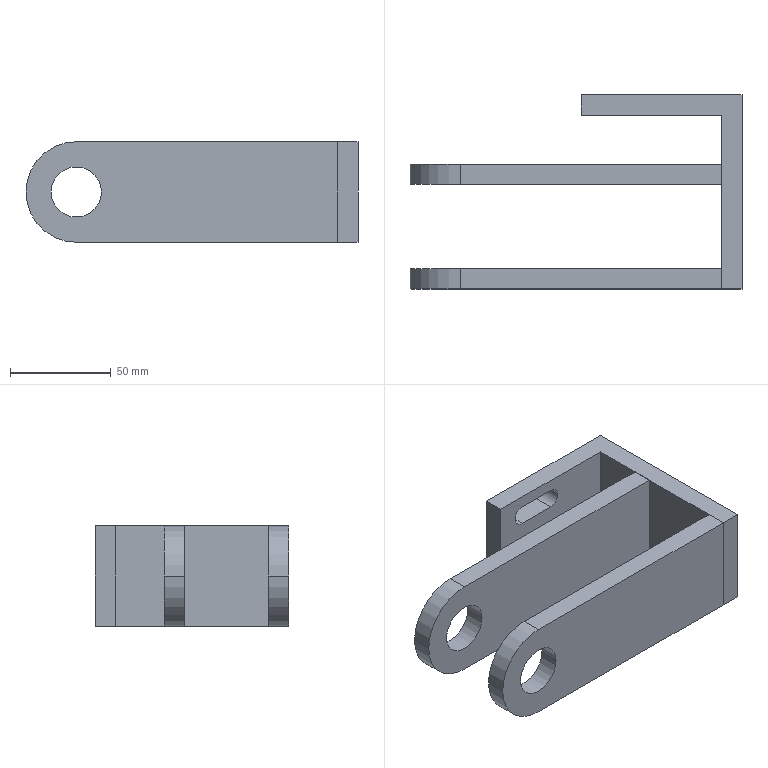Part | SolidWorks | features MoveFace 6, ICE 4, MoveCopyBody 2, Extrusion 1, MirrorSolid 1, Split 1 | 3 solids | 34 faces | box 165 x 96.4 x 50 mm | volume 217447 mm3 | plane 22 | cylinder 12 | commonest cylinder face diameters 10 x4 25 x4 50 x4
STEP:
#1=CARTESIAN_POINT('',(-87.5,-75.,37.));
#2=VERTEX_POINT('',#1);
#3=CARTESIAN_POINT('',(-62.5,-75.,37.));
#4=VERTEX_POINT('',#3);
#5=CARTESIAN_POINT('',(-75.,-75.,37.));
#6=DIRECTION('',(0.,1.,0.));
#7=DIRECTION('',(1.,0.,0.));
#8=AXIS2_PLACEMENT_3D('',#5,#6,#7);
#9=CIRCLE('',#8,12.5);
#10=EDGE_CURVE('',#2,#4,#9,.T.);
#11=ORIENTED_EDGE('',*,*,#10,.T.);
#12=CARTESIAN_POINT('',(-62.5,-85.,37.));
#13=VERTEX_POINT('',#12);
#14=CARTESIAN_POINT('',(-62.5,-75.,37.));
#15=DIRECTION('',(0.,-1.,0.));
#16=VECTOR('',#15,1000.);
#17=LINE('',#14,#16);
#18=EDGE_CURVE('',#4,#13,#17,.T.);
#19=ORIENTED_EDGE('',*,*,#18,.T.);
#20=CARTESIAN_POINT('',(-87.5,-85.,37.));
#21=VERTEX_POINT('',#20);
#22=CARTESIAN_POINT('',(-75.,-85.,37.));
#23=DIRECTION('',(0.,1.,0.));
#24=DIRECTION('',(1.,0.,0.));
#25=AXIS2_PLACEMENT_3D('',#22,#23,#24);
#26=CIRCLE('',#25,12.5);
#27=EDGE_CURVE('',#21,#13,#26,.T.);
#28=ORIENTED_EDGE('',*,*,#27,.F.);
#29=CARTESIAN_POINT('',(-87.5,-75.,37.));
#30=DIRECTION('',(0.,-1.,0.));
#31=VECTOR('',#30,1000.);
#32=LINE('',#29,#31);
#33=EDGE_CURVE('',#2,#21,#32,.T.);
#34=ORIENTED_EDGE('',*,*,#33,.F.);
#35=EDGE_LOOP('',(#11,#19,#28,#34));
#36=FACE_OUTER_BOUND('',#35,.T.);
#37=CARTESIAN_POINT('',(-75.,-75.,37.));
#38=DIRECTION('',(0.,-1.,0.));
#39=DIRECTION('',(-1.,0.,0.));
#40=AXIS2_PLACEMENT_3D('',#37,#38,#39);
#41=CYLINDRICAL_SURFACE('',#40,12.5);
#42=ADVANCED_FACE('',(#36),#41,.F.);
#43=CARTESIAN_POINT('',(-100.,-75.,37.));
#44=VERTEX_POINT('',#43);
#45=CARTESIAN_POINT('',(-75.,-75.,62.));
#46=VERTEX_POINT('',#45);
#47=CARTESIAN_POINT('',(-75.,-75.,37.));
#48=DIRECTION('',(0.,1.,0.));
#49=DIRECTION('',(1.,0.,0.));
#50=AXIS2_PLACEMENT_3D('',#47,#48,#49);
#51=CIRCLE('',#50,25.);
#52=EDGE_CURVE('',#44,#46,#51,.T.);
#53=ORIENTED_EDGE('',*,*,#52,.F.);
#54=CARTESIAN_POINT('',(-100.,-85.,37.));
#55=VERTEX_POINT('',#54);
#56=CARTESIAN_POINT('',(-100.,-75.,37.));
#57=DIRECTION('',(0.,-1.,0.));
#58=VECTOR('',#57,1000.);
#59=LINE('',#56,#58);
#60=EDGE_CURVE('',#44,#55,#59,.T.);
#61=ORIENTED_EDGE('',*,*,#60,.T.);
#62=CARTESIAN_POINT('',(-75.,-85.,62.));
#63=VERTEX_POINT('',#62);
#64=CARTESIAN_POINT('',(-75.,-85.,37.));
#65=DIRECTION('',(0.,1.,0.));
#66=DIRECTION('',(1.,0.,0.));
#67=AXIS2_PLACEMENT_3D('',#64,#65,#66);
#68=CIRCLE('',#67,25.);
#69=EDGE_CURVE('',#55,#63,#68,.T.);
#70=ORIENTED_EDGE('',*,*,#69,.T.);
#71=CARTESIAN_POINT('',(-75.,-75.,62.));
#72=DIRECTION('',(0.,-1.,0.));
#73=VECTOR('',#72,1000.);
#74=LINE('',#71,#73);
#75=EDGE_CURVE('',#46,#63,#74,.T.);
#76=ORIENTED_EDGE('',*,*,#75,.F.);
#77=EDGE_LOOP('',(#53,#61,#70,#76));
#78=FACE_OUTER_BOUND('',#77,.T.);
#79=CARTESIAN_POINT('',(-75.,-75.,37.));
#80=DIRECTION('',(0.,-1.,0.));
#81=DIRECTION('',(-1.,0.,0.));
#82=AXIS2_PLACEMENT_3D('',#79,#80,#81);
#83=CYLINDRICAL_SURFACE('',#82,25.);
#84=ADVANCED_FACE('',(#78),#83,.T.);
#85=CARTESIAN_POINT('',(55.,-85.,12.));
#86=VERTEX_POINT('',#85);
#87=CARTESIAN_POINT('',(55.,-85.,62.));
#88=VERTEX_POINT('',#87);
#89=CARTESIAN_POINT('',(55.,-85.,37.));
#90=DIRECTION('',(0.,0.,1.));
#91=VECTOR('',#90,1000.);
#92=LINE('',#89,#91);
#93=EDGE_CURVE('',#86,#88,#92,.T.);
#94=ORIENTED_EDGE('',*,*,#93,.F.);
#95=CARTESIAN_POINT('',(55.,-75.,12.));
#96=VERTEX_POINT('',#95);
#97=CARTESIAN_POINT('',(55.,-75.,12.));
#98=DIRECTION('',(0.,-1.,0.));
#99=VECTOR('',#98,1000.);
#100=LINE('',#97,#99);
#101=EDGE_CURVE('',#96,#86,#100,.T.);
#102=ORIENTED_EDGE('',*,*,#101,.F.);
#103=CARTESIAN_POINT('',(55.,-75.,62.));
#104=VERTEX_POINT('',#103);
#105=CARTESIAN_POINT('',(55.,-75.,37.));
#106=DIRECTION('',(0.,0.,1.));
#107=VECTOR('',#106,1000.);
#108=LINE('',#105,#107);
#109=EDGE_CURVE('',#96,#104,#108,.T.);
#110=ORIENTED_EDGE('',*,*,#109,.T.);
#111=CARTESIAN_POINT('',(55.,-75.,62.));
#112=DIRECTION('',(0.,1.,0.));
#113=VECTOR('',#112,1000.);
#114=LINE('',#111,#113);
#115=EDGE_CURVE('',#88,#104,#114,.T.);
#116=ORIENTED_EDGE('',*,*,#115,.F.);
#117=EDGE_LOOP('',(#94,#102,#110,#116));
#118=FACE_OUTER_BOUND('',#117,.T.);
#119=CARTESIAN_POINT('',(55.,-85.,-28.));
#120=DIRECTION('',(-1.,0.,0.));
#121=DIRECTION('',(0.,1.,0.));
#122=AXIS2_PLACEMENT_3D('',#119,#120,#121);
#123=PLANE('',#122);
#124=ADVANCED_FACE('',(#118),#123,.F.);
#125=CARTESIAN_POINT('',(-75.,-85.,12.));
#126=VERTEX_POINT('',#125);
#127=CARTESIAN_POINT('',(0.,-85.,12.));
#128=DIRECTION('',(1.,0.,0.));
#129=VECTOR('',#128,1000.);
#130=LINE('',#127,#129);
#131=EDGE_CURVE('',#126,#86,#130,.T.);
#132=ORIENTED_EDGE('',*,*,#131,.T.);
#133=ORIENTED_EDGE('',*,*,#93,.T.);
#134=CARTESIAN_POINT('',(0.,-85.,62.));
#135=DIRECTION('',(1.,0.,0.));
#136=VECTOR('',#135,1000.);
#137=LINE('',#134,#136);
#138=EDGE_CURVE('',#63,#88,#137,.T.);
#139=ORIENTED_EDGE('',*,*,#138,.F.);
#140=ORIENTED_EDGE('',*,*,#69,.F.);
#141=CARTESIAN_POINT('',(-75.,-85.,37.));
#142=DIRECTION('',(0.,1.,0.));
#143=DIRECTION('',(1.,0.,0.));
#144=AXIS2_PLACEMENT_3D('',#141,#142,#143);
#145=CIRCLE('',#144,25.);
#146=EDGE_CURVE('',#126,#55,#145,.T.);
#147=ORIENTED_EDGE('',*,*,#146,.F.);
#148=EDGE_LOOP('',(#132,#133,#139,#140,#147));
#149=FACE_OUTER_BOUND('',#148,.T.);
#150=ORIENTED_EDGE('',*,*,#27,.T.);
#151=CARTESIAN_POINT('',(-75.,-85.,37.));
#152=DIRECTION('',(0.,1.,0.));
#153=DIRECTION('',(1.,0.,0.));
#154=AXIS2_PLACEMENT_3D('',#151,#152,#153);
#155=CIRCLE('',#154,12.5);
#156=EDGE_CURVE('',#13,#21,#155,.T.);
#157=ORIENTED_EDGE('',*,*,#156,.T.);
#158=EDGE_LOOP('',(#150,#157));
#159=FACE_BOUND('',#158,.T.);
#160=CARTESIAN_POINT('',(0.,-85.,37.));
#161=DIRECTION('',(0.,1.,0.));
#162=DIRECTION('',(1.,0.,0.));
#163=AXIS2_PLACEMENT_3D('',#160,#161,#162);
#164=PLANE('',#163);
#165=ADVANCED_FACE('',(#149,#159),#164,.F.);
#166=CARTESIAN_POINT('',(0.,-75.,62.));
#167=DIRECTION('',(1.,0.,0.));
#168=VECTOR('',#167,1000.);
#169=LINE('',#166,#168);
#170=EDGE_CURVE('',#46,#104,#169,.T.);
#171=ORIENTED_EDGE('',*,*,#170,.T.);
#172=ORIENTED_EDGE('',*,*,#109,.F.);
#173=CARTESIAN_POINT('',(-75.,-75.,12.));
#174=VERTEX_POINT('',#173);
#175=CARTESIAN_POINT('',(0.,-75.,12.));
#176=DIRECTION('',(1.,0.,0.));
#177=VECTOR('',#176,1000.);
#178=LINE('',#175,#177);
#179=EDGE_CURVE('',#174,#96,#178,.T.);
#180=ORIENTED_EDGE('',*,*,#179,.F.);
#181=CARTESIAN_POINT('',(-75.,-75.,37.));
#182=DIRECTION('',(0.,1.,0.));
#183=DIRECTION('',(1.,0.,0.));
#184=AXIS2_PLACEMENT_3D('',#181,#182,#183);
#185=CIRCLE('',#184,25.);
#186=EDGE_CURVE('',#174,#44,#185,.T.);
#187=ORIENTED_EDGE('',*,*,#186,.T.);
#188=ORIENTED_EDGE('',*,*,#52,.T.);
#189=EDGE_LOOP('',(#171,#172,#180,#187,#188));
#190=FACE_OUTER_BOUND('',#189,.T.);
#191=ORIENTED_EDGE('',*,*,#10,.F.);
#192=CARTESIAN_POINT('',(-75.,-75.,37.));
#193=DIRECTION('',(0.,1.,0.));
#194=DIRECTION('',(1.,0.,0.));
#195=AXIS2_PLACEMENT_3D('',#192,#193,#194);
#196=CIRCLE('',#195,12.5);
#197=EDGE_CURVE('',#4,#2,#196,.T.);
#198=ORIENTED_EDGE('',*,*,#197,.F.);
#199=EDGE_LOOP('',(#191,#198));
#200=FACE_BOUND('',#199,.T.);
#201=CARTESIAN_POINT('',(0.,-75.,37.));
#202=DIRECTION('',(0.,1.,0.));
#203=DIRECTION('',(1.,0.,0.));
#204=AXIS2_PLACEMENT_3D('',#201,#202,#203);
#205=PLANE('',#204);
#206=ADVANCED_FACE('',(#190,#200),#205,.T.);
#207=ORIENTED_EDGE('',*,*,#18,.F.);
#208=ORIENTED_EDGE('',*,*,#197,.T.);
#209=ORIENTED_EDGE('',*,*,#33,.T.);
#210=ORIENTED_EDGE('',*,*,#156,.F.);
#211=EDGE_LOOP('',(#207,#208,#209,#210));
#212=FACE_OUTER_BOUND('',#211,.T.);
#213=CARTESIAN_POINT('',(-75.,-75.,37.));
#214=DIRECTION('',(0.,-1.,0.));
#215=DIRECTION('',(-1.,0.,0.));
#216=AXIS2_PLACEMENT_3D('',#213,#214,#215);
#217=CYLINDRICAL_SURFACE('',#216,12.5);
#218=ADVANCED_FACE('',(#212),#217,.F.);
#219=ORIENTED_EDGE('',*,*,#60,.F.);
#220=ORIENTED_EDGE('',*,*,#186,.F.);
#221=CARTESIAN_POINT('',(-75.,-75.,12.));
#222=DIRECTION('',(0.,-1.,0.));
#223=VECTOR('',#222,1000.);
#224=LINE('',#221,#223);
#225=EDGE_CURVE('',#174,#126,#224,.T.);
#226=ORIENTED_EDGE('',*,*,#225,.T.);
#227=ORIENTED_EDGE('',*,*,#146,.T.);
#228=EDGE_LOOP('',(#219,#220,#226,#227));
#229=FACE_OUTER_BOUND('',#228,.T.);
#230=CARTESIAN_POINT('',(-75.,-75.,37.));
#231=DIRECTION('',(0.,-1.,0.));
#232=DIRECTION('',(-1.,0.,0.));
#233=AXIS2_PLACEMENT_3D('',#230,#231,#232);
#234=CYLINDRICAL_SURFACE('',#233,25.);
#235=ADVANCED_FACE('',(#229),#234,.T.);
#236=ORIENTED_EDGE('',*,*,#131,.F.);
#237=ORIENTED_EDGE('',*,*,#225,.F.);
#238=ORIENTED_EDGE('',*,*,#179,.T.);
#239=ORIENTED_EDGE('',*,*,#101,.T.);
#240=EDGE_LOOP('',(#236,#237,#238,#239));
#241=FACE_OUTER_BOUND('',#240,.T.);
#242=CARTESIAN_POINT('',(0.,-75.,12.));
#243=DIRECTION('',(0.,0.,-1.));
#244=DIRECTION('',(-1.,0.,0.));
#245=AXIS2_PLACEMENT_3D('',#242,#243,#244);
#246=PLANE('',#245);
#247=ADVANCED_FACE('',(#241),#246,.T.);
#248=ORIENTED_EDGE('',*,*,#138,.T.);
#249=ORIENTED_EDGE('',*,*,#115,.T.);
#250=ORIENTED_EDGE('',*,*,#170,.F.);
#251=ORIENTED_EDGE('',*,*,#75,.T.);
#252=EDGE_LOOP('',(#248,#249,#250,#251));
#253=FACE_OUTER_BOUND('',#252,.T.);
#254=CARTESIAN_POINT('',(0.,-75.,62.));
#255=DIRECTION('',(0.,0.,-1.));
#256=DIRECTION('',(-1.,0.,0.));
#257=AXIS2_PLACEMENT_3D('',#254,#255,#256);
#258=PLANE('',#257);
#259=ADVANCED_FACE('',(#253),#258,.F.);
#260=CLOSED_SHELL('',(#42,#84,#124,#165,#206,#218,#235,#247,#259));
#261=MANIFOLD_SOLID_BREP('',#260);
#262=CARTESIAN_POINT('',(-75.,-33.,12.));
#263=VERTEX_POINT('',#262);
#264=CARTESIAN_POINT('',(-100.,-33.,37.));
#265=VERTEX_POINT('',#264);
#266=CARTESIAN_POINT('',(-75.,-33.,37.));
#267=DIRECTION('',(0.,1.,0.));
#268=DIRECTION('',(1.,0.,0.));
#269=AXIS2_PLACEMENT_3D('',#266,#267,#268);
#270=CIRCLE('',#269,25.);
#271=EDGE_CURVE('',#263,#265,#270,.T.);
#272=ORIENTED_EDGE('',*,*,#271,.T.);
#273=CARTESIAN_POINT('',(-100.,-23.,37.));
#274=VERTEX_POINT('',#273);
#275=CARTESIAN_POINT('',(-100.,-33.,37.));
#276=DIRECTION('',(0.,1.,0.));
#277=VECTOR('',#276,1000.);
#278=LINE('',#275,#277);
#279=EDGE_CURVE('',#265,#274,#278,.T.);
#280=ORIENTED_EDGE('',*,*,#279,.T.);
#281=CARTESIAN_POINT('',(-75.,-23.,12.));
#282=VERTEX_POINT('',#281);
#283=CARTESIAN_POINT('',(-75.,-23.,37.));
#284=DIRECTION('',(0.,1.,0.));
#285=DIRECTION('',(1.,0.,0.));
#286=AXIS2_PLACEMENT_3D('',#283,#284,#285);
#287=CIRCLE('',#286,25.);
#288=EDGE_CURVE('',#282,#274,#287,.T.);
#289=ORIENTED_EDGE('',*,*,#288,.F.);
#290=CARTESIAN_POINT('',(-75.,-33.,12.));
#291=DIRECTION('',(0.,1.,0.));
#292=VECTOR('',#291,1000.);
#293=LINE('',#290,#292);
#294=EDGE_CURVE('',#263,#282,#293,.T.);
#295=ORIENTED_EDGE('',*,*,#294,.F.);
#296=EDGE_LOOP('',(#272,#280,#289,#295));
#297=FACE_OUTER_BOUND('',#296,.T.);
#298=CARTESIAN_POINT('',(-75.,-33.,37.));
#299=DIRECTION('',(0.,1.,0.));
#300=DIRECTION('',(-1.,0.,0.));
#301=AXIS2_PLACEMENT_3D('',#298,#299,#300);
#302=CYLINDRICAL_SURFACE('',#301,25.);
#303=ADVANCED_FACE('',(#297),#302,.T.);
#304=CARTESIAN_POINT('',(-62.5,-33.,37.));
#305=VERTEX_POINT('',#304);
#306=CARTESIAN_POINT('',(-87.5,-33.,37.));
#307=VERTEX_POINT('',#306);
#308=CARTESIAN_POINT('',(-75.,-33.,37.));
#309=DIRECTION('',(0.,1.,0.));
#310=DIRECTION('',(1.,0.,0.));
#311=AXIS2_PLACEMENT_3D('',#308,#309,#310);
#312=CIRCLE('',#311,12.5);
#313=EDGE_CURVE('',#305,#307,#312,.T.);
#314=ORIENTED_EDGE('',*,*,#313,.F.);
#315=CARTESIAN_POINT('',(-62.5,-23.,37.));
#316=VERTEX_POINT('',#315);
#317=CARTESIAN_POINT('',(-62.5,-33.,37.));
#318=DIRECTION('',(0.,1.,0.));
#319=VECTOR('',#318,1000.);
#320=LINE('',#317,#319);
#321=EDGE_CURVE('',#305,#316,#320,.T.);
#322=ORIENTED_EDGE('',*,*,#321,.T.);
#323=CARTESIAN_POINT('',(-87.5,-23.,37.));
#324=VERTEX_POINT('',#323);
#325=CARTESIAN_POINT('',(-75.,-23.,37.));
#326=DIRECTION('',(0.,1.,0.));
#327=DIRECTION('',(1.,0.,0.));
#328=AXIS2_PLACEMENT_3D('',#325,#326,#327);
#329=CIRCLE('',#328,12.5);
#330=EDGE_CURVE('',#316,#324,#329,.T.);
#331=ORIENTED_EDGE('',*,*,#330,.T.);
#332=CARTESIAN_POINT('',(-87.5,-33.,37.));
#333=DIRECTION('',(0.,1.,0.));
#334=VECTOR('',#333,1000.);
#335=LINE('',#332,#334);
#336=EDGE_CURVE('',#307,#324,#335,.T.);
#337=ORIENTED_EDGE('',*,*,#336,.F.);
#338=EDGE_LOOP('',(#314,#322,#331,#337));
#339=FACE_OUTER_BOUND('',#338,.T.);
#340=CARTESIAN_POINT('',(-75.,-33.,37.));
#341=DIRECTION('',(0.,1.,0.));
#342=DIRECTION('',(-1.,0.,0.));
#343=AXIS2_PLACEMENT_3D('',#340,#341,#342);
#344=CYLINDRICAL_SURFACE('',#343,12.5);
#345=ADVANCED_FACE('',(#339),#344,.F.);
#346=CARTESIAN_POINT('',(55.,-33.,62.));
#347=VERTEX_POINT('',#346);
#348=CARTESIAN_POINT('',(55.,-23.,62.));
#349=VERTEX_POINT('',#348);
#350=CARTESIAN_POINT('',(55.,-75.,62.));
#351=DIRECTION('',(0.,1.,0.));
#352=VECTOR('',#351,1000.);
#353=LINE('',#350,#352);
#354=EDGE_CURVE('',#347,#349,#353,.T.);
#355=ORIENTED_EDGE('',*,*,#354,.F.);
#356=CARTESIAN_POINT('',(55.,-33.,12.));
#357=VERTEX_POINT('',#356);
#358=CARTESIAN_POINT('',(55.,-33.,37.));
#359=DIRECTION('',(0.,0.,1.));
#360=VECTOR('',#359,1000.);
#361=LINE('',#358,#360);
#362=EDGE_CURVE('',#357,#347,#361,.T.);
#363=ORIENTED_EDGE('',*,*,#362,.F.);
#364=CARTESIAN_POINT('',(55.,-23.,12.));
#365=VERTEX_POINT('',#364);
#366=CARTESIAN_POINT('',(55.,-33.,12.));
#367=DIRECTION('',(0.,1.,0.));
#368=VECTOR('',#367,1000.);
#369=LINE('',#366,#368);
#370=EDGE_CURVE('',#357,#365,#369,.T.);
#371=ORIENTED_EDGE('',*,*,#370,.T.);
#372=CARTESIAN_POINT('',(55.,-23.,62.));
#373=DIRECTION('',(0.,0.,-1.));
#374=VECTOR('',#373,1000.);
#375=LINE('',#372,#374);
#376=EDGE_CURVE('',#349,#365,#375,.T.);
#377=ORIENTED_EDGE('',*,*,#376,.F.);
#378=EDGE_LOOP('',(#355,#363,#371,#377));
#379=FACE_OUTER_BOUND('',#378,.T.);
#380=CARTESIAN_POINT('',(55.,-85.,-28.));
#381=DIRECTION('',(-1.,0.,0.));
#382=DIRECTION('',(0.,1.,0.));
#383=AXIS2_PLACEMENT_3D('',#380,#381,#382);
#384=PLANE('',#383);
#385=ADVANCED_FACE('',(#379),#384,.F.);
#386=CARTESIAN_POINT('',(-75.,-33.,62.));
#387=VERTEX_POINT('',#386);
#388=CARTESIAN_POINT('',(0.,-33.,62.));
#389=DIRECTION('',(1.,0.,0.));
#390=VECTOR('',#389,1000.);
#391=LINE('',#388,#390);
#392=EDGE_CURVE('',#387,#347,#391,.T.);
#393=ORIENTED_EDGE('',*,*,#392,.F.);
#394=CARTESIAN_POINT('',(-75.,-33.,37.));
#395=DIRECTION('',(0.,1.,0.));
#396=DIRECTION('',(1.,0.,0.));
#397=AXIS2_PLACEMENT_3D('',#394,#395,#396);
#398=CIRCLE('',#397,25.);
#399=EDGE_CURVE('',#265,#387,#398,.T.);
#400=ORIENTED_EDGE('',*,*,#399,.F.);
#401=ORIENTED_EDGE('',*,*,#271,.F.);
#402=CARTESIAN_POINT('',(0.,-33.,12.));
#403=DIRECTION('',(1.,0.,0.));
#404=VECTOR('',#403,1000.);
#405=LINE('',#402,#404);
#406=EDGE_CURVE('',#263,#357,#405,.T.);
#407=ORIENTED_EDGE('',*,*,#406,.T.);
#408=ORIENTED_EDGE('',*,*,#362,.T.);
#409=EDGE_LOOP('',(#393,#400,#401,#407,#408));
#410=FACE_OUTER_BOUND('',#409,.T.);
#411=CARTESIAN_POINT('',(-75.,-33.,37.));
#412=DIRECTION('',(0.,1.,0.));
#413=DIRECTION('',(1.,0.,0.));
#414=AXIS2_PLACEMENT_3D('',#411,#412,#413);
#415=CIRCLE('',#414,12.5);
#416=EDGE_CURVE('',#307,#305,#415,.T.);
#417=ORIENTED_EDGE('',*,*,#416,.T.);
#418=ORIENTED_EDGE('',*,*,#313,.T.);
#419=EDGE_LOOP('',(#417,#418));
#420=FACE_BOUND('',#419,.T.);
#421=CARTESIAN_POINT('',(0.,-33.,37.));
#422=DIRECTION('',(0.,-1.,0.));
#423=DIRECTION('',(1.,0.,0.));
#424=AXIS2_PLACEMENT_3D('',#421,#422,#423);
#425=PLANE('',#424);
#426=ADVANCED_FACE('',(#410,#420),#425,.T.);
#427=ORIENTED_EDGE('',*,*,#392,.T.);
#428=ORIENTED_EDGE('',*,*,#354,.T.);
#429=CARTESIAN_POINT('',(-75.,-23.,62.));
#430=VERTEX_POINT('',#429);
#431=CARTESIAN_POINT('',(85.,-23.,62.));
#432=DIRECTION('',(-1.,0.,0.));
#433=VECTOR('',#432,1000.);
#434=LINE('',#431,#433);
#435=EDGE_CURVE('',#349,#430,#434,.T.);
#436=ORIENTED_EDGE('',*,*,#435,.T.);
#437=CARTESIAN_POINT('',(-75.,-33.,62.));
#438=DIRECTION('',(0.,1.,0.));
#439=VECTOR('',#438,1000.);
#440=LINE('',#437,#439);
#441=EDGE_CURVE('',#387,#430,#440,.T.);
#442=ORIENTED_EDGE('',*,*,#441,.F.);
#443=EDGE_LOOP('',(#427,#428,#436,#442));
#444=FACE_OUTER_BOUND('',#443,.T.);
#445=CARTESIAN_POINT('',(0.,-75.,62.));
#446=DIRECTION('',(0.,0.,-1.));
#447=DIRECTION('',(-1.,0.,0.));
#448=AXIS2_PLACEMENT_3D('',#445,#446,#447);
#449=PLANE('',#448);
#450=ADVANCED_FACE('',(#444),#449,.F.);
#451=ORIENTED_EDGE('',*,*,#279,.F.);
#452=ORIENTED_EDGE('',*,*,#399,.T.);
#453=ORIENTED_EDGE('',*,*,#441,.T.);
#454=CARTESIAN_POINT('',(-75.,-23.,37.));
#455=DIRECTION('',(0.,1.,0.));
#456=DIRECTION('',(1.,0.,0.));
#457=AXIS2_PLACEMENT_3D('',#454,#455,#456);
#458=CIRCLE('',#457,25.);
#459=EDGE_CURVE('',#274,#430,#458,.T.);
#460=ORIENTED_EDGE('',*,*,#459,.F.);
#461=EDGE_LOOP('',(#451,#452,#453,#460));
#462=FACE_OUTER_BOUND('',#461,.T.);
#463=CARTESIAN_POINT('',(-75.,-33.,37.));
#464=DIRECTION('',(0.,1.,0.));
#465=DIRECTION('',(-1.,0.,0.));
#466=AXIS2_PLACEMENT_3D('',#463,#464,#465);
#467=CYLINDRICAL_SURFACE('',#466,25.);
#468=ADVANCED_FACE('',(#462),#467,.T.);
#469=CARTESIAN_POINT('',(0.,-23.,12.));
#470=DIRECTION('',(1.,0.,0.));
#471=VECTOR('',#470,1000.);
#472=LINE('',#469,#471);
#473=EDGE_CURVE('',#282,#365,#472,.T.);
#474=ORIENTED_EDGE('',*,*,#473,.T.);
#475=ORIENTED_EDGE('',*,*,#370,.F.);
#476=ORIENTED_EDGE('',*,*,#406,.F.);
#477=ORIENTED_EDGE('',*,*,#294,.T.);
#478=EDGE_LOOP('',(#474,#475,#476,#477));
#479=FACE_OUTER_BOUND('',#478,.T.);
#480=CARTESIAN_POINT('',(0.,-33.,12.));
#481=DIRECTION('',(0.,0.,-1.));
#482=DIRECTION('',(-1.,0.,0.));
#483=AXIS2_PLACEMENT_3D('',#480,#481,#482);
#484=PLANE('',#483);
#485=ADVANCED_FACE('',(#479),#484,.T.);
#486=ORIENTED_EDGE('',*,*,#321,.F.);
#487=ORIENTED_EDGE('',*,*,#416,.F.);
#488=ORIENTED_EDGE('',*,*,#336,.T.);
#489=CARTESIAN_POINT('',(-75.,-23.,37.));
#490=DIRECTION('',(0.,1.,0.));
#491=DIRECTION('',(1.,0.,0.));
#492=AXIS2_PLACEMENT_3D('',#489,#490,#491);
#493=CIRCLE('',#492,12.5);
#494=EDGE_CURVE('',#324,#316,#493,.T.);
#495=ORIENTED_EDGE('',*,*,#494,.T.);
#496=EDGE_LOOP('',(#486,#487,#488,#495));
#497=FACE_OUTER_BOUND('',#496,.T.);
#498=CARTESIAN_POINT('',(-75.,-33.,37.));
#499=DIRECTION('',(0.,1.,0.));
#500=DIRECTION('',(-1.,0.,0.));
#501=AXIS2_PLACEMENT_3D('',#498,#499,#500);
#502=CYLINDRICAL_SURFACE('',#501,12.5);
#503=ADVANCED_FACE('',(#497),#502,.F.);
#504=ORIENTED_EDGE('',*,*,#494,.F.);
#505=ORIENTED_EDGE('',*,*,#330,.F.);
#506=EDGE_LOOP('',(#504,#505));
#507=FACE_BOUND('',#506,.T.);
#508=ORIENTED_EDGE('',*,*,#435,.F.);
#509=ORIENTED_EDGE('',*,*,#376,.T.);
#510=ORIENTED_EDGE('',*,*,#473,.F.);
#511=ORIENTED_EDGE('',*,*,#288,.T.);
#512=ORIENTED_EDGE('',*,*,#459,.T.);
#513=EDGE_LOOP('',(#508,#509,#510,#511,#512));
#514=FACE_OUTER_BOUND('',#513,.T.);
#515=CARTESIAN_POINT('',(85.,-23.,62.));
#516=DIRECTION('',(0.,-1.,0.));
#517=DIRECTION('',(-1.,0.,0.));
#518=AXIS2_PLACEMENT_3D('',#515,#516,#517);
#519=PLANE('',#518);
#520=ADVANCED_FACE('',(#507,#514),#519,.F.);
#521=CLOSED_SHELL('',(#303,#345,#385,#426,#450,#468,#485,#503,#520));
#522=MANIFOLD_SOLID_BREP('',#521);
#523=CARTESIAN_POINT('',(20.,1.4,18.));
#524=VERTEX_POINT('',#523);
#525=CARTESIAN_POINT('',(0.,1.4,18.));
#526=VERTEX_POINT('',#525);
#527=CARTESIAN_POINT('',(-20.,1.4,18.));
#528=DIRECTION('',(-1.,0.,0.));
#529=VECTOR('',#528,1000.);
#530=LINE('',#527,#529);
#531=EDGE_CURVE('',#524,#526,#530,.T.);
#532=ORIENTED_EDGE('',*,*,#531,.T.);
#533=CARTESIAN_POINT('',(0.,1.4,28.));
#534=VERTEX_POINT('',#533);
#535=CARTESIAN_POINT('',(0.,1.4,23.));
#536=DIRECTION('',(0.,1.,0.));
#537=DIRECTION('',(0.,0.,1.));
#538=AXIS2_PLACEMENT_3D('',#535,#536,#537);
#539=CIRCLE('',#538,5.);
#540=EDGE_CURVE('',#526,#534,#539,.T.);
#541=ORIENTED_EDGE('',*,*,#540,.T.);
#542=CARTESIAN_POINT('',(20.,1.4,28.));
#543=VERTEX_POINT('',#542);
#544=CARTESIAN_POINT('',(-20.,1.4,28.));
#545=DIRECTION('',(1.,0.,0.));
#546=VECTOR('',#545,1000.);
#547=LINE('',#544,#546);
#548=EDGE_CURVE('',#534,#543,#547,.T.);
#549=ORIENTED_EDGE('',*,*,#548,.T.);
#550=CARTESIAN_POINT('',(20.,1.4,23.));
#551=DIRECTION('',(0.,1.,0.));
#552=DIRECTION('',(0.,0.,1.));
#553=AXIS2_PLACEMENT_3D('',#550,#551,#552);
#554=CIRCLE('',#553,5.);
#555=EDGE_CURVE('',#543,#524,#554,.T.);
#556=ORIENTED_EDGE('',*,*,#555,.T.);
#557=EDGE_LOOP('',(#532,#541,#549,#556));
#558=FACE_BOUND('',#557,.T.);
#559=CARTESIAN_POINT('',(20.,1.4,46.));
#560=VERTEX_POINT('',#559);
#561=CARTESIAN_POINT('',(0.,1.4,46.));
#562=VERTEX_POINT('',#561);
#563=CARTESIAN_POINT('',(0.,1.4,46.));
#564=DIRECTION('',(-1.,0.,0.));
#565=VECTOR('',#564,1000.);
#566=LINE('',#563,#565);
#567=EDGE_CURVE('',#560,#562,#566,.T.);
#568=ORIENTED_EDGE('',*,*,#567,.T.);
#569=CARTESIAN_POINT('',(0.,1.4,56.));
#570=VERTEX_POINT('',#569);
#571=CARTESIAN_POINT('',(0.,1.4,51.));
#572=DIRECTION('',(0.,1.,0.));
#573=DIRECTION('',(0.,0.,1.));
#574=AXIS2_PLACEMENT_3D('',#571,#572,#573);
#575=CIRCLE('',#574,5.);
#576=EDGE_CURVE('',#562,#570,#575,.T.);
#577=ORIENTED_EDGE('',*,*,#576,.T.);
#578=CARTESIAN_POINT('',(20.,1.4,56.));
#579=VERTEX_POINT('',#578);
#580=CARTESIAN_POINT('',(0.,1.4,56.));
#581=DIRECTION('',(1.,0.,0.));
#582=VECTOR('',#581,1000.);
#583=LINE('',#580,#582);
#584=EDGE_CURVE('',#570,#579,#583,.T.);
#585=ORIENTED_EDGE('',*,*,#584,.T.);
#586=CARTESIAN_POINT('',(20.,1.4,51.));
#587=DIRECTION('',(0.,1.,0.));
#588=DIRECTION('',(0.,0.,1.));
#589=AXIS2_PLACEMENT_3D('',#586,#587,#588);
#590=CIRCLE('',#589,5.);
#591=EDGE_CURVE('',#579,#560,#590,.T.);
#592=ORIENTED_EDGE('',*,*,#591,.T.);
#593=EDGE_LOOP('',(#568,#577,#585,#592));
#594=FACE_BOUND('',#593,.T.);
#595=CARTESIAN_POINT('',(55.,1.4,12.));
#596=VERTEX_POINT('',#595);
#597=CARTESIAN_POINT('',(-15.,1.4,12.));
#598=VERTEX_POINT('',#597);
#599=CARTESIAN_POINT('',(-15.,1.4,12.));
#600=DIRECTION('',(-1.,0.,0.));
#601=VECTOR('',#600,1000.);
#602=LINE('',#599,#601);
#603=EDGE_CURVE('',#596,#598,#602,.T.);
#604=ORIENTED_EDGE('',*,*,#603,.F.);
#605=CARTESIAN_POINT('',(55.,1.4,62.));
#606=VERTEX_POINT('',#605);
#607=CARTESIAN_POINT('',(55.,1.4,0.));
#608=DIRECTION('',(0.,0.,1.));
#609=VECTOR('',#608,1000.);
#610=LINE('',#607,#609);
#611=EDGE_CURVE('',#596,#606,#610,.T.);
#612=ORIENTED_EDGE('',*,*,#611,.T.);
#613=CARTESIAN_POINT('',(-15.,1.4,62.));
#614=VERTEX_POINT('',#613);
#615=CARTESIAN_POINT('',(-15.,1.4,62.));
#616=DIRECTION('',(1.,0.,0.));
#617=VECTOR('',#616,1000.);
#618=LINE('',#615,#617);
#619=EDGE_CURVE('',#614,#606,#618,.T.);
#620=ORIENTED_EDGE('',*,*,#619,.F.);
#621=CARTESIAN_POINT('',(-15.,1.4,0.));
#622=DIRECTION('',(0.,0.,1.));
#623=VECTOR('',#622,1000.);
#624=LINE('',#621,#623);
#625=EDGE_CURVE('',#598,#614,#624,.T.);
#626=ORIENTED_EDGE('',*,*,#625,.F.);
#627=EDGE_LOOP('',(#604,#612,#620,#626));
#628=FACE_OUTER_BOUND('',#627,.T.);
#629=CARTESIAN_POINT('',(-20.,1.4,0.));
#630=DIRECTION('',(0.,1.,0.));
#631=DIRECTION('',(0.,0.,1.));
#632=AXIS2_PLACEMENT_3D('',#629,#630,#631);
#633=PLANE('',#632);
#634=ADVANCED_FACE('',(#558,#594,#628),#633,.F.);
#635=CARTESIAN_POINT('',(20.,11.4,46.));
#636=VERTEX_POINT('',#635);
#637=CARTESIAN_POINT('',(0.,11.4,46.));
#638=VERTEX_POINT('',#637);
#639=CARTESIAN_POINT('',(0.,11.4,46.));
#640=DIRECTION('',(-1.,0.,0.));
#641=VECTOR('',#640,1000.);
#642=LINE('',#639,#641);
#643=EDGE_CURVE('',#636,#638,#642,.T.);
#644=ORIENTED_EDGE('',*,*,#643,.T.);
#645=CARTESIAN_POINT('',(0.,1.4,46.));
#646=DIRECTION('',(0.,1.,0.));
#647=VECTOR('',#646,1000.);
#648=LINE('',#645,#647);
#649=EDGE_CURVE('',#562,#638,#648,.T.);
#650=ORIENTED_EDGE('',*,*,#649,.F.);
#651=ORIENTED_EDGE('',*,*,#567,.F.);
#652=CARTESIAN_POINT('',(20.,1.4,46.));
#653=DIRECTION('',(0.,1.,0.));
#654=VECTOR('',#653,1000.);
#655=LINE('',#652,#654);
#656=EDGE_CURVE('',#560,#636,#655,.T.);
#657=ORIENTED_EDGE('',*,*,#656,.T.);
#658=EDGE_LOOP('',(#644,#650,#651,#657));
#659=FACE_OUTER_BOUND('',#658,.T.);
#660=CARTESIAN_POINT('',(0.,1.4,46.));
#661=DIRECTION('',(0.,0.,-1.));
#662=DIRECTION('',(-1.,0.,0.));
#663=AXIS2_PLACEMENT_3D('',#660,#661,#662);
#664=PLANE('',#663);
#665=ADVANCED_FACE('',(#659),#664,.F.);
#666=CARTESIAN_POINT('',(0.,11.4,56.));
#667=VERTEX_POINT('',#666);
#668=CARTESIAN_POINT('',(0.,11.4,51.));
#669=DIRECTION('',(0.,1.,0.));
#670=DIRECTION('',(0.,0.,1.));
#671=AXIS2_PLACEMENT_3D('',#668,#669,#670);
#672=CIRCLE('',#671,5.);
#673=EDGE_CURVE('',#638,#667,#672,.T.);
#674=ORIENTED_EDGE('',*,*,#673,.T.);
#675=CARTESIAN_POINT('',(0.,1.4,56.));
#676=DIRECTION('',(0.,1.,0.));
#677=VECTOR('',#676,1000.);
#678=LINE('',#675,#677);
#679=EDGE_CURVE('',#570,#667,#678,.T.);
#680=ORIENTED_EDGE('',*,*,#679,.F.);
#681=ORIENTED_EDGE('',*,*,#576,.F.);
#682=ORIENTED_EDGE('',*,*,#649,.T.);
#683=EDGE_LOOP('',(#674,#680,#681,#682));
#684=FACE_OUTER_BOUND('',#683,.T.);
#685=CARTESIAN_POINT('',(0.,1.4,51.));
#686=DIRECTION('',(0.,1.,0.));
#687=DIRECTION('',(0.,0.,1.));
#688=AXIS2_PLACEMENT_3D('',#685,#686,#687);
#689=CYLINDRICAL_SURFACE('',#688,5.);
#690=ADVANCED_FACE('',(#684),#689,.F.);
#691=CARTESIAN_POINT('',(20.,11.4,56.));
#692=VERTEX_POINT('',#691);
#693=CARTESIAN_POINT('',(0.,11.4,56.));
#694=DIRECTION('',(1.,0.,0.));
#695=VECTOR('',#694,1000.);
#696=LINE('',#693,#695);
#697=EDGE_CURVE('',#667,#692,#696,.T.);
#698=ORIENTED_EDGE('',*,*,#697,.T.);
#699=CARTESIAN_POINT('',(20.,1.4,56.));
#700=DIRECTION('',(0.,1.,0.));
#701=VECTOR('',#700,1000.);
#702=LINE('',#699,#701);
#703=EDGE_CURVE('',#579,#692,#702,.T.);
#704=ORIENTED_EDGE('',*,*,#703,.F.);
#705=ORIENTED_EDGE('',*,*,#584,.F.);
#706=ORIENTED_EDGE('',*,*,#679,.T.);
#707=EDGE_LOOP('',(#698,#704,#705,#706));
#708=FACE_OUTER_BOUND('',#707,.T.);
#709=CARTESIAN_POINT('',(0.,1.4,56.));
#710=DIRECTION('',(0.,0.,1.));
#711=DIRECTION('',(1.,0.,0.));
#712=AXIS2_PLACEMENT_3D('',#709,#710,#711);
#713=PLANE('',#712);
#714=ADVANCED_FACE('',(#708),#713,.F.);
#715=CARTESIAN_POINT('',(20.,11.4,51.));
#716=DIRECTION('',(0.,1.,0.));
#717=DIRECTION('',(0.,0.,1.));
#718=AXIS2_PLACEMENT_3D('',#715,#716,#717);
#719=CIRCLE('',#718,5.);
#720=EDGE_CURVE('',#692,#636,#719,.T.);
#721=ORIENTED_EDGE('',*,*,#720,.T.);
#722=ORIENTED_EDGE('',*,*,#656,.F.);
#723=ORIENTED_EDGE('',*,*,#591,.F.);
#724=ORIENTED_EDGE('',*,*,#703,.T.);
#725=EDGE_LOOP('',(#721,#722,#723,#724));
#726=FACE_OUTER_BOUND('',#725,.T.);
#727=CARTESIAN_POINT('',(20.,1.4,51.));
#728=DIRECTION('',(0.,1.,0.));
#729=DIRECTION('',(0.,0.,1.));
#730=AXIS2_PLACEMENT_3D('',#727,#728,#729);
#731=CYLINDRICAL_SURFACE('',#730,5.);
#732=ADVANCED_FACE('',(#726),#731,.F.);
#733=CARTESIAN_POINT('',(65.,11.4,12.));
#734=VERTEX_POINT('',#733);
#735=CARTESIAN_POINT('',(-15.,11.4,12.));
#736=VERTEX_POINT('',#735);
#737=CARTESIAN_POINT('',(65.,11.4,12.));
#738=DIRECTION('',(-1.,0.,0.));
#739=VECTOR('',#738,1000.);
#740=LINE('',#737,#739);
#741=EDGE_CURVE('',#734,#736,#740,.T.);
#742=ORIENTED_EDGE('',*,*,#741,.F.);
#743=CARTESIAN_POINT('',(65.,-85.,12.));
#744=VERTEX_POINT('',#743);
#745=CARTESIAN_POINT('',(65.,-88.6,12.));
#746=DIRECTION('',(0.,1.,0.));
#747=VECTOR('',#746,1000.);
#748=LINE('',#745,#747);
#749=EDGE_CURVE('',#744,#734,#748,.T.);
#750=ORIENTED_EDGE('',*,*,#749,.F.);
#751=CARTESIAN_POINT('',(55.,-85.,12.));
#752=VERTEX_POINT('',#751);
#753=CARTESIAN_POINT('',(-20.,-85.,12.));
#754=DIRECTION('',(1.,0.,0.));
#755=VECTOR('',#754,1000.);
#756=LINE('',#753,#755);
#757=EDGE_CURVE('',#752,#744,#756,.T.);
#758=ORIENTED_EDGE('',*,*,#757,.F.);
#759=CARTESIAN_POINT('',(55.,-63.6,12.));
#760=DIRECTION('',(0.,-1.,0.));
#761=VECTOR('',#760,1000.);
#762=LINE('',#759,#761);
#763=EDGE_CURVE('',#596,#752,#762,.T.);
#764=ORIENTED_EDGE('',*,*,#763,.F.);
#765=ORIENTED_EDGE('',*,*,#603,.T.);
#766=CARTESIAN_POINT('',(-15.,1.4,12.));
#767=DIRECTION('',(0.,1.,0.));
#768=VECTOR('',#767,1000.);
#769=LINE('',#766,#768);
#770=EDGE_CURVE('',#598,#736,#769,.T.);
#771=ORIENTED_EDGE('',*,*,#770,.T.);
#772=EDGE_LOOP('',(#742,#750,#758,#764,#765,#771));
#773=FACE_OUTER_BOUND('',#772,.T.);
#774=CARTESIAN_POINT('',(-20.,-63.6,12.));
#775=DIRECTION('',(0.,0.,1.));
#776=DIRECTION('',(1.,0.,0.));
#777=AXIS2_PLACEMENT_3D('',#774,#775,#776);
#778=PLANE('',#777);
#779=ADVANCED_FACE('',(#773),#778,.F.);
#780=CARTESIAN_POINT('',(65.,11.4,62.));
#781=VERTEX_POINT('',#780);
#782=CARTESIAN_POINT('',(65.,-85.,62.));
#783=VERTEX_POINT('',#782);
#784=CARTESIAN_POINT('',(65.,-88.6,62.));
#785=DIRECTION('',(0.,-1.,0.));
#786=VECTOR('',#785,1000.);
#787=LINE('',#784,#786);
#788=EDGE_CURVE('',#781,#783,#787,.T.);
#789=ORIENTED_EDGE('',*,*,#788,.F.);
#790=CARTESIAN_POINT('',(-15.,11.4,62.));
#791=VERTEX_POINT('',#790);
#792=CARTESIAN_POINT('',(65.,11.4,62.));
#793=DIRECTION('',(-1.,0.,0.));
#794=VECTOR('',#793,1000.);
#795=LINE('',#792,#794);
#796=EDGE_CURVE('',#781,#791,#795,.T.);
#797=ORIENTED_EDGE('',*,*,#796,.T.);
#798=CARTESIAN_POINT('',(-15.,1.4,62.));
#799=DIRECTION('',(0.,1.,0.));
#800=VECTOR('',#799,1000.);
#801=LINE('',#798,#800);
#802=EDGE_CURVE('',#614,#791,#801,.T.);
#803=ORIENTED_EDGE('',*,*,#802,.F.);
#804=ORIENTED_EDGE('',*,*,#619,.T.);
#805=CARTESIAN_POINT('',(55.,-85.,62.));
#806=VERTEX_POINT('',#805);
#807=CARTESIAN_POINT('',(55.,-88.6,62.));
#808=DIRECTION('',(0.,1.,0.));
#809=VECTOR('',#808,1000.);
#810=LINE('',#807,#809);
#811=EDGE_CURVE('',#806,#606,#810,.T.);
#812=ORIENTED_EDGE('',*,*,#811,.F.);
#813=CARTESIAN_POINT('',(-20.,-85.,62.));
#814=DIRECTION('',(-1.,0.,0.));
#815=VECTOR('',#814,1000.);
#816=LINE('',#813,#815);
#817=EDGE_CURVE('',#783,#806,#816,.T.);
#818=ORIENTED_EDGE('',*,*,#817,.F.);
#819=EDGE_LOOP('',(#789,#797,#803,#804,#812,#818));
#820=FACE_OUTER_BOUND('',#819,.T.);
#821=CARTESIAN_POINT('',(65.,-88.6,62.));
#822=DIRECTION('',(0.,0.,-1.));
#823=DIRECTION('',(-1.,0.,0.));
#824=AXIS2_PLACEMENT_3D('',#821,#822,#823);
#825=PLANE('',#824);
#826=ADVANCED_FACE('',(#820),#825,.F.);
#827=CARTESIAN_POINT('',(-15.,11.4,0.));
#828=DIRECTION('',(0.,0.,1.));
#829=VECTOR('',#828,1000.);
#830=LINE('',#827,#829);
#831=EDGE_CURVE('',#736,#791,#830,.T.);
#832=ORIENTED_EDGE('',*,*,#831,.F.);
#833=ORIENTED_EDGE('',*,*,#770,.F.);
#834=ORIENTED_EDGE('',*,*,#625,.T.);
#835=ORIENTED_EDGE('',*,*,#802,.T.);
#836=EDGE_LOOP('',(#832,#833,#834,#835));
#837=FACE_OUTER_BOUND('',#836,.T.);
#838=CARTESIAN_POINT('',(-15.,1.4,0.));
#839=DIRECTION('',(-1.,0.,0.));
#840=DIRECTION('',(0.,0.,1.));
#841=AXIS2_PLACEMENT_3D('',#838,#839,#840);
#842=PLANE('',#841);
#843=ADVANCED_FACE('',(#837),#842,.T.);
#844=CARTESIAN_POINT('',(0.,11.4,28.));
#845=VERTEX_POINT('',#844);
#846=CARTESIAN_POINT('',(20.,11.4,28.));
#847=VERTEX_POINT('',#846);
#848=CARTESIAN_POINT('',(0.,11.4,28.));
#849=DIRECTION('',(1.,0.,0.));
#850=VECTOR('',#849,1000.);
#851=LINE('',#848,#850);
#852=EDGE_CURVE('',#845,#847,#851,.T.);
#853=ORIENTED_EDGE('',*,*,#852,.F.);
#854=CARTESIAN_POINT('',(0.,11.4,18.));
#855=VERTEX_POINT('',#854);
#856=CARTESIAN_POINT('',(0.,11.4,23.));
#857=DIRECTION('',(0.,1.,0.));
#858=DIRECTION('',(0.,0.,1.));
#859=AXIS2_PLACEMENT_3D('',#856,#857,#858);
#860=CIRCLE('',#859,5.);
#861=EDGE_CURVE('',#855,#845,#860,.T.);
#862=ORIENTED_EDGE('',*,*,#861,.F.);
#863=CARTESIAN_POINT('',(20.,11.4,18.));
#864=VERTEX_POINT('',#863);
#865=CARTESIAN_POINT('',(0.,11.4,18.));
#866=DIRECTION('',(-1.,0.,0.));
#867=VECTOR('',#866,1000.);
#868=LINE('',#865,#867);
#869=EDGE_CURVE('',#864,#855,#868,.T.);
#870=ORIENTED_EDGE('',*,*,#869,.F.);
#871=CARTESIAN_POINT('',(20.,11.4,23.));
#872=DIRECTION('',(0.,1.,0.));
#873=DIRECTION('',(0.,0.,1.));
#874=AXIS2_PLACEMENT_3D('',#871,#872,#873);
#875=CIRCLE('',#874,5.);
#876=EDGE_CURVE('',#847,#864,#875,.T.);
#877=ORIENTED_EDGE('',*,*,#876,.F.);
#878=EDGE_LOOP('',(#853,#862,#870,#877));
#879=FACE_BOUND('',#878,.T.);
#880=ORIENTED_EDGE('',*,*,#796,.F.);
#881=CARTESIAN_POINT('',(65.,11.4,62.));
#882=DIRECTION('',(0.,0.,-1.));
#883=VECTOR('',#882,1000.);
#884=LINE('',#881,#883);
#885=EDGE_CURVE('',#781,#734,#884,.T.);
#886=ORIENTED_EDGE('',*,*,#885,.T.);
#887=ORIENTED_EDGE('',*,*,#741,.T.);
#888=ORIENTED_EDGE('',*,*,#831,.T.);
#889=EDGE_LOOP('',(#880,#886,#887,#888));
#890=FACE_OUTER_BOUND('',#889,.T.);
#891=ORIENTED_EDGE('',*,*,#673,.F.);
#892=ORIENTED_EDGE('',*,*,#643,.F.);
#893=ORIENTED_EDGE('',*,*,#720,.F.);
#894=ORIENTED_EDGE('',*,*,#697,.F.);
#895=EDGE_LOOP('',(#891,#892,#893,#894));
#896=FACE_BOUND('',#895,.T.);
#897=CARTESIAN_POINT('',(65.,11.4,0.));
#898=DIRECTION('',(0.,-1.,0.));
#899=DIRECTION('',(0.,0.,-1.));
#900=AXIS2_PLACEMENT_3D('',#897,#898,#899);
#901=PLANE('',#900);
#902=ADVANCED_FACE('',(#879,#890,#896),#901,.F.);
#903=ORIENTED_EDGE('',*,*,#749,.T.);
#904=ORIENTED_EDGE('',*,*,#885,.F.);
#905=ORIENTED_EDGE('',*,*,#788,.T.);
#906=CARTESIAN_POINT('',(65.,-85.,0.));
#907=DIRECTION('',(0.,0.,-1.));
#908=VECTOR('',#907,1000.);
#909=LINE('',#906,#908);
#910=EDGE_CURVE('',#783,#744,#909,.T.);
#911=ORIENTED_EDGE('',*,*,#910,.T.);
#912=EDGE_LOOP('',(#903,#904,#905,#911));
#913=FACE_OUTER_BOUND('',#912,.T.);
#914=CARTESIAN_POINT('',(65.,0.,0.));
#915=DIRECTION('',(1.,0.,0.));
#916=DIRECTION('',(0.,0.,-1.));
#917=AXIS2_PLACEMENT_3D('',#914,#915,#916);
#918=PLANE('',#917);
#919=ADVANCED_FACE('',(#913),#918,.T.);
#920=CARTESIAN_POINT('',(55.,-85.,10.));
#921=DIRECTION('',(0.,0.,1.));
#922=VECTOR('',#921,1000.);
#923=LINE('',#920,#922);
#924=EDGE_CURVE('',#752,#806,#923,.T.);
#925=ORIENTED_EDGE('',*,*,#924,.F.);
#926=ORIENTED_EDGE('',*,*,#757,.T.);
#927=ORIENTED_EDGE('',*,*,#910,.F.);
#928=ORIENTED_EDGE('',*,*,#817,.T.);
#929=EDGE_LOOP('',(#925,#926,#927,#928));
#930=FACE_OUTER_BOUND('',#929,.T.);
#931=CARTESIAN_POINT('',(-20.,-85.,10.));
#932=DIRECTION('',(0.,1.,0.));
#933=DIRECTION('',(-1.,0.,0.));
#934=AXIS2_PLACEMENT_3D('',#931,#932,#933);
#935=PLANE('',#934);
#936=ADVANCED_FACE('',(#930),#935,.F.);
#937=ORIENTED_EDGE('',*,*,#924,.T.);
#938=ORIENTED_EDGE('',*,*,#811,.T.);
#939=ORIENTED_EDGE('',*,*,#611,.F.);
#940=ORIENTED_EDGE('',*,*,#763,.T.);
#941=EDGE_LOOP('',(#937,#938,#939,#940));
#942=FACE_OUTER_BOUND('',#941,.T.);
#943=CARTESIAN_POINT('',(55.,65.,0.));
#944=DIRECTION('',(-1.,0.,0.));
#945=DIRECTION('',(0.,0.,1.));
#946=AXIS2_PLACEMENT_3D('',#943,#944,#945);
#947=PLANE('',#946);
#948=ADVANCED_FACE('',(#942),#947,.T.);
#949=CARTESIAN_POINT('',(0.,-8.6,18.));
#950=DIRECTION('',(0.,1.,0.));
#951=VECTOR('',#950,1000.);
#952=LINE('',#949,#951);
#953=EDGE_CURVE('',#526,#855,#952,.T.);
#954=ORIENTED_EDGE('',*,*,#953,.T.);
#955=ORIENTED_EDGE('',*,*,#861,.T.);
#956=CARTESIAN_POINT('',(0.,-8.6,28.));
#957=DIRECTION('',(0.,1.,0.));
#958=VECTOR('',#957,1000.);
#959=LINE('',#956,#958);
#960=EDGE_CURVE('',#534,#845,#959,.T.);
#961=ORIENTED_EDGE('',*,*,#960,.F.);
#962=ORIENTED_EDGE('',*,*,#540,.F.);
#963=EDGE_LOOP('',(#954,#955,#961,#962));
#964=FACE_OUTER_BOUND('',#963,.T.);
#965=CARTESIAN_POINT('',(0.,-8.6,23.));
#966=DIRECTION('',(0.,1.,0.));
#967=DIRECTION('',(0.,0.,1.));
#968=AXIS2_PLACEMENT_3D('',#965,#966,#967);
#969=CYLINDRICAL_SURFACE('',#968,5.);
#970=ADVANCED_FACE('',(#964),#969,.F.);
#971=CARTESIAN_POINT('',(20.,-8.6,18.));
#972=DIRECTION('',(0.,1.,0.));
#973=VECTOR('',#972,1000.);
#974=LINE('',#971,#973);
#975=EDGE_CURVE('',#524,#864,#974,.T.);
#976=ORIENTED_EDGE('',*,*,#975,.T.);
#977=ORIENTED_EDGE('',*,*,#869,.T.);
#978=ORIENTED_EDGE('',*,*,#953,.F.);
#979=ORIENTED_EDGE('',*,*,#531,.F.);
#980=EDGE_LOOP('',(#976,#977,#978,#979));
#981=FACE_OUTER_BOUND('',#980,.T.);
#982=CARTESIAN_POINT('',(0.,-8.6,18.));
#983=DIRECTION('',(0.,0.,-1.));
#984=DIRECTION('',(-1.,0.,0.));
#985=AXIS2_PLACEMENT_3D('',#982,#983,#984);
#986=PLANE('',#985);
#987=ADVANCED_FACE('',(#981),#986,.F.);
#988=CARTESIAN_POINT('',(20.,-8.6,28.));
#989=DIRECTION('',(0.,1.,0.));
#990=VECTOR('',#989,1000.);
#991=LINE('',#988,#990);
#992=EDGE_CURVE('',#543,#847,#991,.T.);
#993=ORIENTED_EDGE('',*,*,#992,.T.);
#994=ORIENTED_EDGE('',*,*,#876,.T.);
#995=ORIENTED_EDGE('',*,*,#975,.F.);
#996=ORIENTED_EDGE('',*,*,#555,.F.);
#997=EDGE_LOOP('',(#993,#994,#995,#996));
#998=FACE_OUTER_BOUND('',#997,.T.);
#999=CARTESIAN_POINT('',(20.,-8.6,23.));
#1000=DIRECTION('',(0.,1.,0.));
#1001=DIRECTION('',(0.,0.,1.));
#1002=AXIS2_PLACEMENT_3D('',#999,#1000,#1001);
#1003=CYLINDRICAL_SURFACE('',#1002,5.);
#1004=ADVANCED_FACE('',(#998),#1003,.F.);
#1005=ORIENTED_EDGE('',*,*,#960,.T.);
#1006=ORIENTED_EDGE('',*,*,#852,.T.);
#1007=ORIENTED_EDGE('',*,*,#992,.F.);
#1008=ORIENTED_EDGE('',*,*,#548,.F.);
#1009=EDGE_LOOP('',(#1005,#1006,#1007,#1008));
#1010=FACE_OUTER_BOUND('',#1009,.T.);
#1011=CARTESIAN_POINT('',(0.,-8.6,28.));
#1012=DIRECTION('',(0.,0.,1.));
#1013=DIRECTION('',(1.,0.,0.));
#1014=AXIS2_PLACEMENT_3D('',#1011,#1012,#1013);
#1015=PLANE('',#1014);
#1016=ADVANCED_FACE('',(#1010),#1015,.F.);
#1017=CLOSED_SHELL('',(#634,#665,#690,#714,#732,#779,#826,#843,#902,#919,#936,#948,#970,#987,#1004,#1016));
#1018=MANIFOLD_SOLID_BREP('',#1017);
#1019=CARTESIAN_POINT('',(0.,0.,0.));
#1020=DIRECTION('',(0.,0.,1.));
#1021=DIRECTION('',(1.,0.,0.));
#1022=AXIS2_PLACEMENT_3D('',#1019,#1020,#1021);
#1023=(LENGTH_UNIT()NAMED_UNIT(*)SI_UNIT(.MILLI.,.METRE.));
#1024=UNCERTAINTY_MEASURE_WITH_UNIT(LENGTH_MEASURE(0.00001),#1023,'','');
#1025=(NAMED_UNIT(*)PLANE_ANGLE_UNIT()SI_UNIT($,.RADIAN.));
#1026=(NAMED_UNIT(*)SI_UNIT($,.STERADIAN.)SOLID_ANGLE_UNIT());
#1027=(GEOMETRIC_REPRESENTATION_CONTEXT(3)GLOBAL_UNCERTAINTY_ASSIGNED_CONTEXT((#1024))GLOBAL_UNIT_ASSIGNED_CONTEXT((#1023,#1025,#1026))REPRESENTATION_CONTEXT('',''));
#1028=ADVANCED_BREP_SHAPE_REPRESENTATION('',(#261,#522,#1018,#1022),#1027);